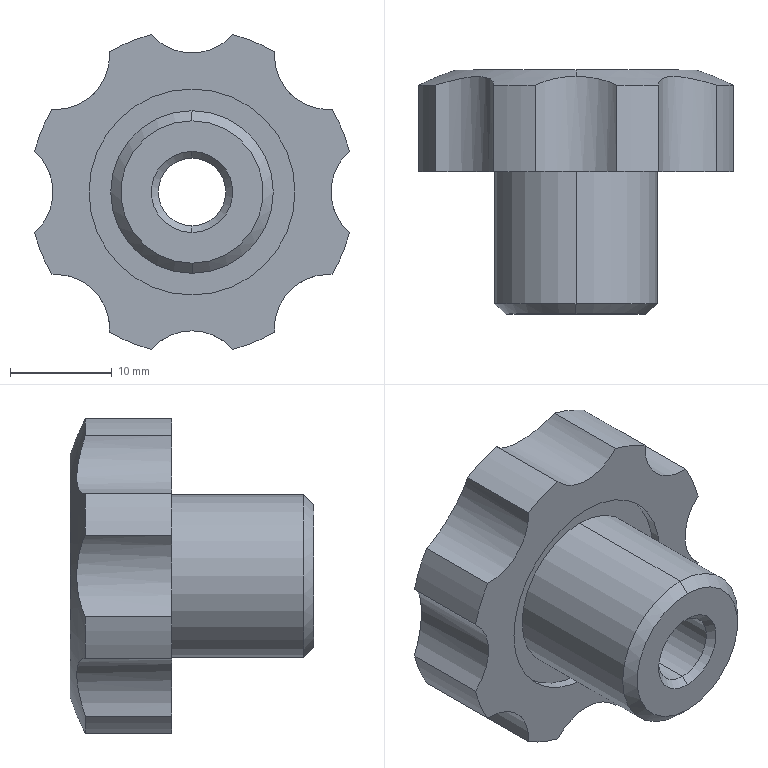Part | STEP file | 1 solid | 41 faces | box 30.977 x 24 x 30.977 mm | volume 8556 mm3 | cylinder 29 | plane 6 | cone 6 | commonest cylinder face diameters 10.667 x11 32 x8 16 x4 20.267 x4 6.647 x2